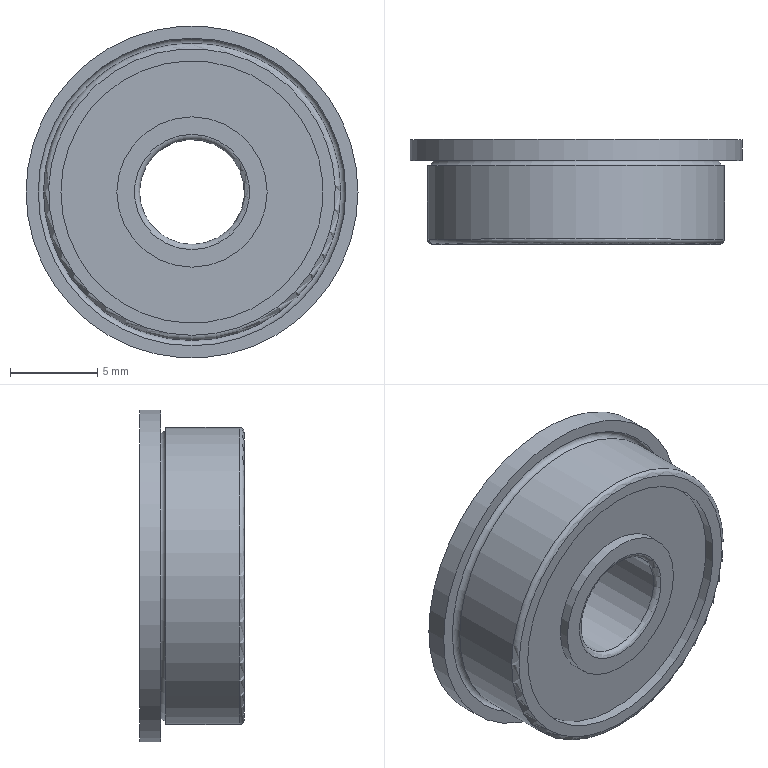Part | STEP file | ROTATION MC_NEW VER-0610_519 | 1 solid | 18 faces | box 19 x 6 x 19 mm | volume 1113 mm3 | plane 7 | cylinder 7 | torus 4 | commonest cylinder face diameters 8.6 x2 15 x2 6 x1 17 x1 19 x1
STEP:
#1=CARTESIAN_POINT('',(-272.021,581.268,-79.291));
#2=VERTEX_POINT('',#1);
#3=CARTESIAN_POINT('',(-272.021,581.268,-71.091));
#4=DIRECTION('',(0.,1.,0.));
#5=DIRECTION('',(0.,0.,-1.));
#6=AXIS2_PLACEMENT_3D('',#3,#4,#5);
#7=CIRCLE('',#6,8.2);
#8=EDGE_CURVE('',#2,#2,#7,.T.);
#9=ORIENTED_EDGE('',*,*,#8,.F.);
#10=EDGE_LOOP('',(#9));
#11=FACE_OUTER_BOUND('',#10,.T.);
#12=CARTESIAN_POINT('',(-279.521,581.268,-71.091));
#13=VERTEX_POINT('',#12);
#14=CARTESIAN_POINT('',(-272.021,581.268,-71.091));
#15=DIRECTION('',(0.,1.,0.));
#16=DIRECTION('',(0.,0.,-1.));
#17=AXIS2_PLACEMENT_3D('',#14,#15,#16);
#18=CIRCLE('',#17,7.5);
#19=EDGE_CURVE('',#13,#13,#18,.T.);
#20=ORIENTED_EDGE('',*,*,#19,.T.);
#21=EDGE_LOOP('',(#20));
#22=FACE_BOUND('',#21,.T.);
#23=CARTESIAN_POINT('',(-280.221,581.268,-71.091));
#24=DIRECTION('',(0.,-1.,0.));
#25=DIRECTION('',(0.,0.,-1.));
#26=AXIS2_PLACEMENT_3D('',#23,#24,#25);
#27=PLANE('',#26);
#28=ADVANCED_FACE('',(#11,#22),#27,.T.);
#29=CARTESIAN_POINT('',(-276.321,581.833,-71.091));
#30=VERTEX_POINT('',#29);
#31=CARTESIAN_POINT('',(-272.021,581.833,-71.091));
#32=DIRECTION('',(0.,1.,0.));
#33=DIRECTION('',(0.,0.,-1.));
#34=AXIS2_PLACEMENT_3D('',#31,#32,#33);
#35=CIRCLE('',#34,4.3);
#36=EDGE_CURVE('',#30,#30,#35,.T.);
#37=ORIENTED_EDGE('',*,*,#36,.F.);
#38=CARTESIAN_POINT('',(-276.321,581.268,-71.091));
#39=VERTEX_POINT('',#38);
#40=CARTESIAN_POINT('',(-276.321,581.551,-71.091));
#41=DIRECTION('',(0.,-1.,0.));
#42=VECTOR('',#41,4.3);
#43=LINE('',#40,#42);
#44=EDGE_CURVE('',#30,#39,#43,.T.);
#45=ORIENTED_EDGE('',*,*,#44,.T.);
#46=CARTESIAN_POINT('',(-272.021,581.268,-71.091));
#47=DIRECTION('',(0.,1.,0.));
#48=DIRECTION('',(0.,0.,-1.));
#49=AXIS2_PLACEMENT_3D('',#46,#47,#48);
#50=CIRCLE('',#49,4.3);
#51=EDGE_CURVE('',#39,#39,#50,.T.);
#52=ORIENTED_EDGE('',*,*,#51,.T.);
#53=ORIENTED_EDGE('',*,*,#44,.F.);
#54=EDGE_LOOP('',(#37,#45,#52,#53));
#55=FACE_OUTER_BOUND('',#54,.T.);
#56=CARTESIAN_POINT('',(-272.021,581.551,-71.091));
#57=DIRECTION('',(0.,1.,0.));
#58=DIRECTION('',(1.,0.,0.));
#59=AXIS2_PLACEMENT_3D('',#56,#57,#58);
#60=CYLINDRICAL_SURFACE('',#59,4.3);
#61=ADVANCED_FACE('',(#55),#60,.T.);
#62=ORIENTED_EDGE('',*,*,#19,.F.);
#63=CARTESIAN_POINT('',(-279.521,581.833,-71.091));
#64=VERTEX_POINT('',#63);
#65=CARTESIAN_POINT('',(-279.521,581.551,-71.091));
#66=DIRECTION('',(0.,1.,0.));
#67=VECTOR('',#66,7.5);
#68=LINE('',#65,#67);
#69=EDGE_CURVE('',#13,#64,#68,.T.);
#70=ORIENTED_EDGE('',*,*,#69,.T.);
#71=CARTESIAN_POINT('',(-272.021,581.833,-71.091));
#72=DIRECTION('',(0.,1.,0.));
#73=DIRECTION('',(0.,0.,-1.));
#74=AXIS2_PLACEMENT_3D('',#71,#72,#73);
#75=CIRCLE('',#74,7.5);
#76=EDGE_CURVE('',#64,#64,#75,.T.);
#77=ORIENTED_EDGE('',*,*,#76,.T.);
#78=ORIENTED_EDGE('',*,*,#69,.F.);
#79=EDGE_LOOP('',(#62,#70,#77,#78));
#80=FACE_OUTER_BOUND('',#79,.T.);
#81=CARTESIAN_POINT('',(-272.021,581.551,-71.091));
#82=DIRECTION('',(0.,1.,0.));
#83=DIRECTION('',(1.,0.,0.));
#84=AXIS2_PLACEMENT_3D('',#81,#82,#83);
#85=CYLINDRICAL_SURFACE('',#84,7.5);
#86=ADVANCED_FACE('',(#80),#85,.F.);
#87=CARTESIAN_POINT('',(-272.021,586.068,-79.891));
#88=VERTEX_POINT('',#87);
#89=CARTESIAN_POINT('',(-272.021,586.068,-71.091));
#90=DIRECTION('',(0.,1.,0.));
#91=DIRECTION('',(0.,0.,-1.));
#92=AXIS2_PLACEMENT_3D('',#89,#90,#91);
#93=CIRCLE('',#92,8.8);
#94=EDGE_CURVE('',#88,#88,#93,.T.);
#95=ORIENTED_EDGE('',*,*,#94,.F.);
#96=CARTESIAN_POINT('',(-272.021,585.768,-79.591));
#97=VERTEX_POINT('',#96);
#98=CARTESIAN_POINT('',(-272.021,586.068,-79.591));
#99=DIRECTION('',(1.,0.,0.));
#100=DIRECTION('',(0.,0.,-1.));
#101=AXIS2_PLACEMENT_3D('',#98,#99,#100);
#102=CIRCLE('',#101,0.3);
#103=EDGE_CURVE('',#88,#97,#102,.T.);
#104=ORIENTED_EDGE('',*,*,#103,.T.);
#105=CARTESIAN_POINT('',(-280.521,585.768,-71.091));
#106=VERTEX_POINT('',#105);
#107=CARTESIAN_POINT('',(-272.021,585.768,-71.091));
#108=DIRECTION('',(0.,1.,0.));
#109=DIRECTION('',(0.,0.,-1.));
#110=AXIS2_PLACEMENT_3D('',#107,#108,#109);
#111=CIRCLE('',#110,8.5);
#112=EDGE_CURVE('',#97,#106,#111,.T.);
#113=ORIENTED_EDGE('',*,*,#112,.T.);
#114=CARTESIAN_POINT('',(-272.021,585.768,-71.091));
#115=DIRECTION('',(0.,1.,0.));
#116=DIRECTION('',(0.,0.,-1.));
#117=AXIS2_PLACEMENT_3D('',#114,#115,#116);
#118=CIRCLE('',#117,8.5);
#119=EDGE_CURVE('',#106,#97,#118,.T.);
#120=ORIENTED_EDGE('',*,*,#119,.T.);
#121=ORIENTED_EDGE('',*,*,#103,.F.);
#122=EDGE_LOOP('',(#95,#104,#113,#120,#121));
#123=FACE_OUTER_BOUND('',#122,.T.);
#124=CARTESIAN_POINT('',(-272.021,586.068,-71.091));
#125=DIRECTION('',(0.,1.,0.));
#126=DIRECTION('',(0.,0.,1.));
#127=AXIS2_PLACEMENT_3D('',#124,#125,#126);
#128=TOROIDAL_SURFACE('',#127,8.5,0.3);
#129=ADVANCED_FACE('',(#123),#128,.F.);
#130=CARTESIAN_POINT('',(-276.321,587.268,-71.091));
#131=VERTEX_POINT('',#130);
#132=CARTESIAN_POINT('',(-272.021,587.268,-71.091));
#133=DIRECTION('',(0.,1.,0.));
#134=DIRECTION('',(0.,0.,-1.));
#135=AXIS2_PLACEMENT_3D('',#132,#133,#134);
#136=CIRCLE('',#135,4.3);
#137=EDGE_CURVE('',#131,#131,#136,.T.);
#138=ORIENTED_EDGE('',*,*,#137,.F.);
#139=CARTESIAN_POINT('',(-276.321,586.703,-71.091));
#140=VERTEX_POINT('',#139);
#141=CARTESIAN_POINT('',(-276.321,586.986,-71.091));
#142=DIRECTION('',(0.,-1.,0.));
#143=VECTOR('',#142,4.3);
#144=LINE('',#141,#143);
#145=EDGE_CURVE('',#131,#140,#144,.T.);
#146=ORIENTED_EDGE('',*,*,#145,.T.);
#147=CARTESIAN_POINT('',(-272.021,586.703,-71.091));
#148=DIRECTION('',(0.,1.,0.));
#149=DIRECTION('',(0.,0.,-1.));
#150=AXIS2_PLACEMENT_3D('',#147,#148,#149);
#151=CIRCLE('',#150,4.3);
#152=EDGE_CURVE('',#140,#140,#151,.T.);
#153=ORIENTED_EDGE('',*,*,#152,.T.);
#154=ORIENTED_EDGE('',*,*,#145,.F.);
#155=EDGE_LOOP('',(#138,#146,#153,#154));
#156=FACE_OUTER_BOUND('',#155,.T.);
#157=CARTESIAN_POINT('',(-272.021,586.986,-71.091));
#158=DIRECTION('',(0.,1.,0.));
#159=DIRECTION('',(1.,0.,0.));
#160=AXIS2_PLACEMENT_3D('',#157,#158,#159);
#161=CYLINDRICAL_SURFACE('',#160,4.3);
#162=ADVANCED_FACE('',(#156),#161,.T.);
#163=ORIENTED_EDGE('',*,*,#51,.F.);
#164=EDGE_LOOP('',(#163));
#165=FACE_OUTER_BOUND('',#164,.T.);
#166=CARTESIAN_POINT('',(-272.021,581.268,-74.391));
#167=VERTEX_POINT('',#166);
#168=CARTESIAN_POINT('',(-272.021,581.268,-71.091));
#169=DIRECTION('',(0.,1.,0.));
#170=DIRECTION('',(0.,0.,-1.));
#171=AXIS2_PLACEMENT_3D('',#168,#169,#170);
#172=CIRCLE('',#171,3.3);
#173=EDGE_CURVE('',#167,#167,#172,.T.);
#174=ORIENTED_EDGE('',*,*,#173,.T.);
#175=EDGE_LOOP('',(#174));
#176=FACE_BOUND('',#175,.T.);
#177=CARTESIAN_POINT('',(-276.321,581.268,-71.091));
#178=DIRECTION('',(0.,-1.,0.));
#179=DIRECTION('',(0.,0.,-1.));
#180=AXIS2_PLACEMENT_3D('',#177,#178,#179);
#181=PLANE('',#180);
#182=ADVANCED_FACE('',(#165,#176),#181,.T.);
#183=CARTESIAN_POINT('',(-280.521,581.568,-71.091));
#184=VERTEX_POINT('',#183);
#185=CARTESIAN_POINT('',(-272.021,581.568,-79.591));
#186=VERTEX_POINT('',#185);
#187=CARTESIAN_POINT('',(-272.021,581.568,-71.091));
#188=DIRECTION('',(0.,1.,0.));
#189=DIRECTION('',(0.,0.,-1.));
#190=AXIS2_PLACEMENT_3D('',#187,#188,#189);
#191=CIRCLE('',#190,8.5);
#192=EDGE_CURVE('',#184,#186,#191,.T.);
#193=ORIENTED_EDGE('',*,*,#192,.F.);
#194=CARTESIAN_POINT('',(-272.021,581.568,-71.091));
#195=DIRECTION('',(0.,1.,0.));
#196=DIRECTION('',(0.,0.,-1.));
#197=AXIS2_PLACEMENT_3D('',#194,#195,#196);
#198=CIRCLE('',#197,8.5);
#199=EDGE_CURVE('',#186,#184,#198,.T.);
#200=ORIENTED_EDGE('',*,*,#199,.F.);
#201=CARTESIAN_POINT('',(-272.021,581.568,-79.291));
#202=DIRECTION('',(-1.,0.,0.));
#203=DIRECTION('',(0.,0.,-1.));
#204=AXIS2_PLACEMENT_3D('',#201,#202,#203);
#205=CIRCLE('',#204,0.3);
#206=EDGE_CURVE('',#186,#2,#205,.T.);
#207=ORIENTED_EDGE('',*,*,#206,.T.);
#208=ORIENTED_EDGE('',*,*,#8,.T.);
#209=ORIENTED_EDGE('',*,*,#206,.F.);
#210=EDGE_LOOP('',(#193,#200,#207,#208,#209));
#211=FACE_OUTER_BOUND('',#210,.T.);
#212=CARTESIAN_POINT('',(-272.021,581.568,-71.091));
#213=DIRECTION('',(0.,1.,0.));
#214=DIRECTION('',(0.,0.,1.));
#215=AXIS2_PLACEMENT_3D('',#212,#213,#214);
#216=TOROIDAL_SURFACE('',#215,8.2,0.3);
#217=ADVANCED_FACE('',(#211),#216,.T.);
#218=CARTESIAN_POINT('',(-275.021,586.968,-71.091));
#219=VERTEX_POINT('',#218);
#220=CARTESIAN_POINT('',(-272.021,586.968,-74.091));
#221=VERTEX_POINT('',#220);
#222=CARTESIAN_POINT('',(-272.021,586.968,-71.091));
#223=DIRECTION('',(0.,1.,0.));
#224=DIRECTION('',(0.,0.,-1.));
#225=AXIS2_PLACEMENT_3D('',#222,#223,#224);
#226=CIRCLE('',#225,3.);
#227=EDGE_CURVE('',#219,#221,#226,.T.);
#228=ORIENTED_EDGE('',*,*,#227,.F.);
#229=CARTESIAN_POINT('',(-272.021,586.968,-71.091));
#230=DIRECTION('',(0.,1.,0.));
#231=DIRECTION('',(0.,0.,-1.));
#232=AXIS2_PLACEMENT_3D('',#229,#230,#231);
#233=CIRCLE('',#232,3.);
#234=EDGE_CURVE('',#221,#219,#233,.T.);
#235=ORIENTED_EDGE('',*,*,#234,.F.);
#236=CARTESIAN_POINT('',(-272.021,587.268,-74.391));
#237=VERTEX_POINT('',#236);
#238=CARTESIAN_POINT('',(-272.021,586.968,-74.391));
#239=DIRECTION('',(-1.,0.,0.));
#240=DIRECTION('',(0.,0.,-1.));
#241=AXIS2_PLACEMENT_3D('',#238,#239,#240);
#242=CIRCLE('',#241,0.3);
#243=EDGE_CURVE('',#221,#237,#242,.T.);
#244=ORIENTED_EDGE('',*,*,#243,.T.);
#245=CARTESIAN_POINT('',(-272.021,587.268,-71.091));
#246=DIRECTION('',(0.,1.,0.));
#247=DIRECTION('',(0.,0.,-1.));
#248=AXIS2_PLACEMENT_3D('',#245,#246,#247);
#249=CIRCLE('',#248,3.3);
#250=EDGE_CURVE('',#237,#237,#249,.T.);
#251=ORIENTED_EDGE('',*,*,#250,.T.);
#252=ORIENTED_EDGE('',*,*,#243,.F.);
#253=EDGE_LOOP('',(#228,#235,#244,#251,#252));
#254=FACE_OUTER_BOUND('',#253,.T.);
#255=CARTESIAN_POINT('',(-272.021,586.968,-71.091));
#256=DIRECTION('',(0.,1.,0.));
#257=DIRECTION('',(0.,0.,1.));
#258=AXIS2_PLACEMENT_3D('',#255,#256,#257);
#259=TOROIDAL_SURFACE('',#258,3.3,0.3);
#260=ADVANCED_FACE('',(#254),#259,.T.);
#261=ORIENTED_EDGE('',*,*,#76,.F.);
#262=EDGE_LOOP('',(#261));
#263=FACE_OUTER_BOUND('',#262,.T.);
#264=ORIENTED_EDGE('',*,*,#36,.T.);
#265=EDGE_LOOP('',(#264));
#266=FACE_BOUND('',#265,.T.);
#267=CARTESIAN_POINT('',(-279.521,581.833,-71.091));
#268=DIRECTION('',(0.,-1.,0.));
#269=DIRECTION('',(0.,0.,-1.));
#270=AXIS2_PLACEMENT_3D('',#267,#268,#269);
#271=PLANE('',#270);
#272=ADVANCED_FACE('',(#263,#266),#271,.T.);
#273=CARTESIAN_POINT('',(-279.521,586.703,-71.091));
#274=VERTEX_POINT('',#273);
#275=CARTESIAN_POINT('',(-272.021,586.703,-71.091));
#276=DIRECTION('',(0.,1.,0.));
#277=DIRECTION('',(0.,0.,-1.));
#278=AXIS2_PLACEMENT_3D('',#275,#276,#277);
#279=CIRCLE('',#278,7.5);
#280=EDGE_CURVE('',#274,#274,#279,.T.);
#281=ORIENTED_EDGE('',*,*,#280,.F.);
#282=CARTESIAN_POINT('',(-279.521,587.268,-71.091));
#283=VERTEX_POINT('',#282);
#284=CARTESIAN_POINT('',(-279.521,586.986,-71.091));
#285=DIRECTION('',(0.,1.,0.));
#286=VECTOR('',#285,7.5);
#287=LINE('',#284,#286);
#288=EDGE_CURVE('',#274,#283,#287,.T.);
#289=ORIENTED_EDGE('',*,*,#288,.T.);
#290=CARTESIAN_POINT('',(-272.021,587.268,-71.091));
#291=DIRECTION('',(0.,1.,0.));
#292=DIRECTION('',(0.,0.,-1.));
#293=AXIS2_PLACEMENT_3D('',#290,#291,#292);
#294=CIRCLE('',#293,7.5);
#295=EDGE_CURVE('',#283,#283,#294,.T.);
#296=ORIENTED_EDGE('',*,*,#295,.T.);
#297=ORIENTED_EDGE('',*,*,#288,.F.);
#298=EDGE_LOOP('',(#281,#289,#296,#297));
#299=FACE_OUTER_BOUND('',#298,.T.);
#300=CARTESIAN_POINT('',(-272.021,586.986,-71.091));
#301=DIRECTION('',(0.,1.,0.));
#302=DIRECTION('',(1.,0.,0.));
#303=AXIS2_PLACEMENT_3D('',#300,#301,#302);
#304=CYLINDRICAL_SURFACE('',#303,7.5);
#305=ADVANCED_FACE('',(#299),#304,.F.);
#306=CARTESIAN_POINT('',(-281.521,587.268,-71.091));
#307=VERTEX_POINT('',#306);
#308=CARTESIAN_POINT('',(-272.021,587.268,-71.091));
#309=DIRECTION('',(0.,1.,0.));
#310=DIRECTION('',(0.,0.,-1.));
#311=AXIS2_PLACEMENT_3D('',#308,#309,#310);
#312=CIRCLE('',#311,9.5);
#313=EDGE_CURVE('',#307,#307,#312,.T.);
#314=ORIENTED_EDGE('',*,*,#313,.F.);
#315=CARTESIAN_POINT('',(-281.521,586.068,-71.091));
#316=VERTEX_POINT('',#315);
#317=CARTESIAN_POINT('',(-281.521,586.668,-71.091));
#318=DIRECTION('',(0.,-1.,0.));
#319=VECTOR('',#318,9.5);
#320=LINE('',#317,#319);
#321=EDGE_CURVE('',#307,#316,#320,.T.);
#322=ORIENTED_EDGE('',*,*,#321,.T.);
#323=CARTESIAN_POINT('',(-272.021,586.068,-71.091));
#324=DIRECTION('',(0.,1.,0.));
#325=DIRECTION('',(0.,0.,-1.));
#326=AXIS2_PLACEMENT_3D('',#323,#324,#325);
#327=CIRCLE('',#326,9.5);
#328=EDGE_CURVE('',#316,#316,#327,.T.);
#329=ORIENTED_EDGE('',*,*,#328,.T.);
#330=ORIENTED_EDGE('',*,*,#321,.F.);
#331=EDGE_LOOP('',(#314,#322,#329,#330));
#332=FACE_OUTER_BOUND('',#331,.T.);
#333=CARTESIAN_POINT('',(-272.021,586.668,-71.091));
#334=DIRECTION('',(0.,1.,0.));
#335=DIRECTION('',(1.,0.,0.));
#336=AXIS2_PLACEMENT_3D('',#333,#334,#335);
#337=CYLINDRICAL_SURFACE('',#336,9.5);
#338=ADVANCED_FACE('',(#332),#337,.T.);
#339=ORIENTED_EDGE('',*,*,#328,.F.);
#340=EDGE_LOOP('',(#339));
#341=FACE_OUTER_BOUND('',#340,.T.);
#342=ORIENTED_EDGE('',*,*,#94,.T.);
#343=EDGE_LOOP('',(#342));
#344=FACE_BOUND('',#343,.T.);
#345=CARTESIAN_POINT('',(-281.521,586.068,-71.091));
#346=DIRECTION('',(0.,-1.,0.));
#347=DIRECTION('',(0.,0.,-1.));
#348=AXIS2_PLACEMENT_3D('',#345,#346,#347);
#349=PLANE('',#348);
#350=ADVANCED_FACE('',(#341,#344),#349,.T.);
#351=CARTESIAN_POINT('',(-272.021,581.568,-74.091));
#352=VERTEX_POINT('',#351);
#353=CARTESIAN_POINT('',(-275.021,581.568,-71.091));
#354=VERTEX_POINT('',#353);
#355=CARTESIAN_POINT('',(-272.021,581.568,-71.091));
#356=DIRECTION('',(0.,1.,0.));
#357=DIRECTION('',(0.,0.,-1.));
#358=AXIS2_PLACEMENT_3D('',#355,#356,#357);
#359=CIRCLE('',#358,3.);
#360=EDGE_CURVE('',#352,#354,#359,.T.);
#361=ORIENTED_EDGE('',*,*,#360,.F.);
#362=CARTESIAN_POINT('',(-272.021,581.568,-71.091));
#363=DIRECTION('',(0.,1.,0.));
#364=DIRECTION('',(0.,0.,-1.));
#365=AXIS2_PLACEMENT_3D('',#362,#363,#364);
#366=CIRCLE('',#365,3.);
#367=EDGE_CURVE('',#354,#352,#366,.T.);
#368=ORIENTED_EDGE('',*,*,#367,.F.);
#369=CARTESIAN_POINT('',(-275.021,584.268,-71.091));
#370=DIRECTION('',(0.,1.,0.));
#371=VECTOR('',#370,3.);
#372=LINE('',#369,#371);
#373=EDGE_CURVE('',#354,#219,#372,.T.);
#374=ORIENTED_EDGE('',*,*,#373,.T.);
#375=ORIENTED_EDGE('',*,*,#227,.T.);
#376=ORIENTED_EDGE('',*,*,#234,.T.);
#377=ORIENTED_EDGE('',*,*,#373,.F.);
#378=EDGE_LOOP('',(#361,#368,#374,#375,#376,#377));
#379=FACE_OUTER_BOUND('',#378,.T.);
#380=CARTESIAN_POINT('',(-272.021,584.268,-71.091));
#381=DIRECTION('',(0.,1.,0.));
#382=DIRECTION('',(1.,0.,0.));
#383=AXIS2_PLACEMENT_3D('',#380,#381,#382);
#384=CYLINDRICAL_SURFACE('',#383,3.);
#385=ADVANCED_FACE('',(#379),#384,.F.);
#386=ORIENTED_EDGE('',*,*,#173,.F.);
#387=CARTESIAN_POINT('',(-272.021,581.568,-74.391));
#388=DIRECTION('',(-1.,0.,0.));
#389=DIRECTION('',(0.,0.,-1.));
#390=AXIS2_PLACEMENT_3D('',#387,#388,#389);
#391=CIRCLE('',#390,0.3);
#392=EDGE_CURVE('',#167,#352,#391,.T.);
#393=ORIENTED_EDGE('',*,*,#392,.T.);
#394=ORIENTED_EDGE('',*,*,#360,.T.);
#395=ORIENTED_EDGE('',*,*,#367,.T.);
#396=ORIENTED_EDGE('',*,*,#392,.F.);
#397=EDGE_LOOP('',(#386,#393,#394,#395,#396));
#398=FACE_OUTER_BOUND('',#397,.T.);
#399=CARTESIAN_POINT('',(-272.021,581.568,-71.091));
#400=DIRECTION('',(0.,1.,0.));
#401=DIRECTION('',(0.,0.,1.));
#402=AXIS2_PLACEMENT_3D('',#399,#400,#401);
#403=TOROIDAL_SURFACE('',#402,3.3,0.3);
#404=ADVANCED_FACE('',(#398),#403,.T.);
#405=ORIENTED_EDGE('',*,*,#119,.F.);
#406=CARTESIAN_POINT('',(-280.521,583.668,-71.091));
#407=DIRECTION('',(0.,-1.,0.));
#408=VECTOR('',#407,8.5);
#409=LINE('',#406,#408);
#410=EDGE_CURVE('',#106,#184,#409,.T.);
#411=ORIENTED_EDGE('',*,*,#410,.T.);
#412=ORIENTED_EDGE('',*,*,#192,.T.);
#413=ORIENTED_EDGE('',*,*,#199,.T.);
#414=ORIENTED_EDGE('',*,*,#410,.F.);
#415=ORIENTED_EDGE('',*,*,#112,.F.);
#416=EDGE_LOOP('',(#405,#411,#412,#413,#414,#415));
#417=FACE_OUTER_BOUND('',#416,.T.);
#418=CARTESIAN_POINT('',(-272.021,583.668,-71.091));
#419=DIRECTION('',(0.,1.,0.));
#420=DIRECTION('',(1.,0.,0.));
#421=AXIS2_PLACEMENT_3D('',#418,#419,#420);
#422=CYLINDRICAL_SURFACE('',#421,8.5);
#423=ADVANCED_FACE('',(#417),#422,.T.);
#424=ORIENTED_EDGE('',*,*,#137,.T.);
#425=EDGE_LOOP('',(#424));
#426=FACE_OUTER_BOUND('',#425,.T.);
#427=ORIENTED_EDGE('',*,*,#250,.F.);
#428=EDGE_LOOP('',(#427));
#429=FACE_BOUND('',#428,.T.);
#430=CARTESIAN_POINT('',(-275.321,587.268,-71.091));
#431=DIRECTION('',(0.,1.,0.));
#432=DIRECTION('',(0.,0.,1.));
#433=AXIS2_PLACEMENT_3D('',#430,#431,#432);
#434=PLANE('',#433);
#435=ADVANCED_FACE('',(#426,#429),#434,.T.);
#436=ORIENTED_EDGE('',*,*,#313,.T.);
#437=EDGE_LOOP('',(#436));
#438=FACE_OUTER_BOUND('',#437,.T.);
#439=ORIENTED_EDGE('',*,*,#295,.F.);
#440=EDGE_LOOP('',(#439));
#441=FACE_BOUND('',#440,.T.);
#442=CARTESIAN_POINT('',(-279.521,587.268,-71.091));
#443=DIRECTION('',(0.,1.,0.));
#444=DIRECTION('',(0.,0.,1.));
#445=AXIS2_PLACEMENT_3D('',#442,#443,#444);
#446=PLANE('',#445);
#447=ADVANCED_FACE('',(#438,#441),#446,.T.);
#448=ORIENTED_EDGE('',*,*,#280,.T.);
#449=EDGE_LOOP('',(#448));
#450=FACE_OUTER_BOUND('',#449,.T.);
#451=ORIENTED_EDGE('',*,*,#152,.F.);
#452=EDGE_LOOP('',(#451));
#453=FACE_BOUND('',#452,.T.);
#454=CARTESIAN_POINT('',(-276.321,586.703,-71.091));
#455=DIRECTION('',(0.,1.,0.));
#456=DIRECTION('',(0.,0.,1.));
#457=AXIS2_PLACEMENT_3D('',#454,#455,#456);
#458=PLANE('',#457);
#459=ADVANCED_FACE('',(#450,#453),#458,.T.);
#460=CLOSED_SHELL('',(#28,#61,#86,#129,#162,#182,#217,#260,#272,#305,#338,#350,#385,#404,#423,#435,#447,#459));
#461=MANIFOLD_SOLID_BREP('',#460);
#462=(LENGTH_UNIT()NAMED_UNIT(*)SI_UNIT(.MILLI.,.METRE.));
#463=UNCERTAINTY_MEASURE_WITH_UNIT(LENGTH_MEASURE(0.01),#462,'','');
#464=(NAMED_UNIT(*)PLANE_ANGLE_UNIT()SI_UNIT($,.RADIAN.));
#465=(NAMED_UNIT(*)SI_UNIT($,.STERADIAN.)SOLID_ANGLE_UNIT());
#466=(GEOMETRIC_REPRESENTATION_CONTEXT(3)GLOBAL_UNCERTAINTY_ASSIGNED_CONTEXT((#463))GLOBAL_UNIT_ASSIGNED_CONTEXT((#462,#464,#465))REPRESENTATION_CONTEXT('',''));
#467=ADVANCED_BREP_SHAPE_REPRESENTATION('',(#461),#466);